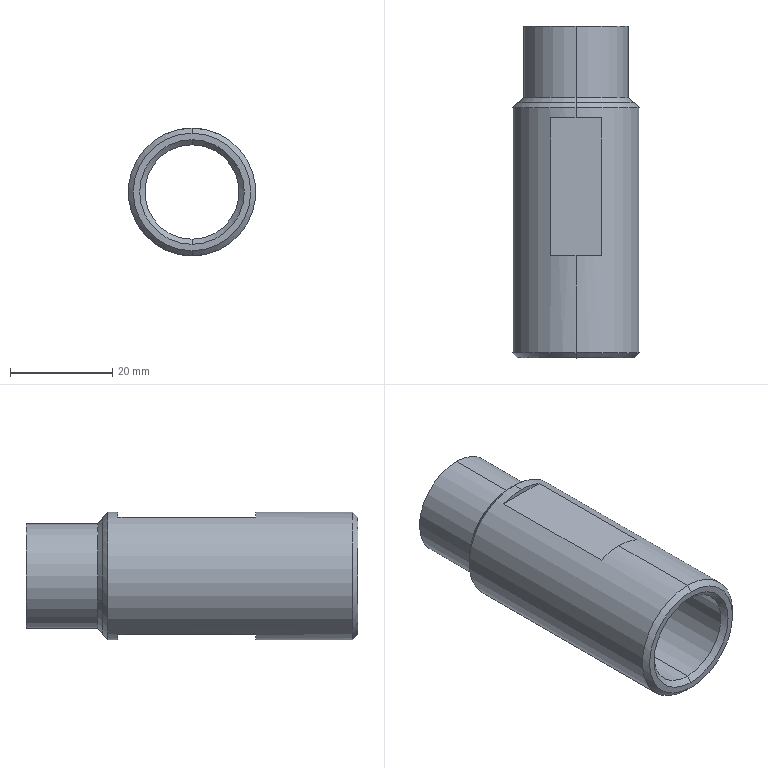Part | STEP file | 1 solid | 24 faces | box 25 x 65 x 25 mm | volume 11563 mm3 | cone 10 | plane 8 | cylinder 6 | commonest cylinder face diameters 18.5 x2 20.5 x2 25 x2